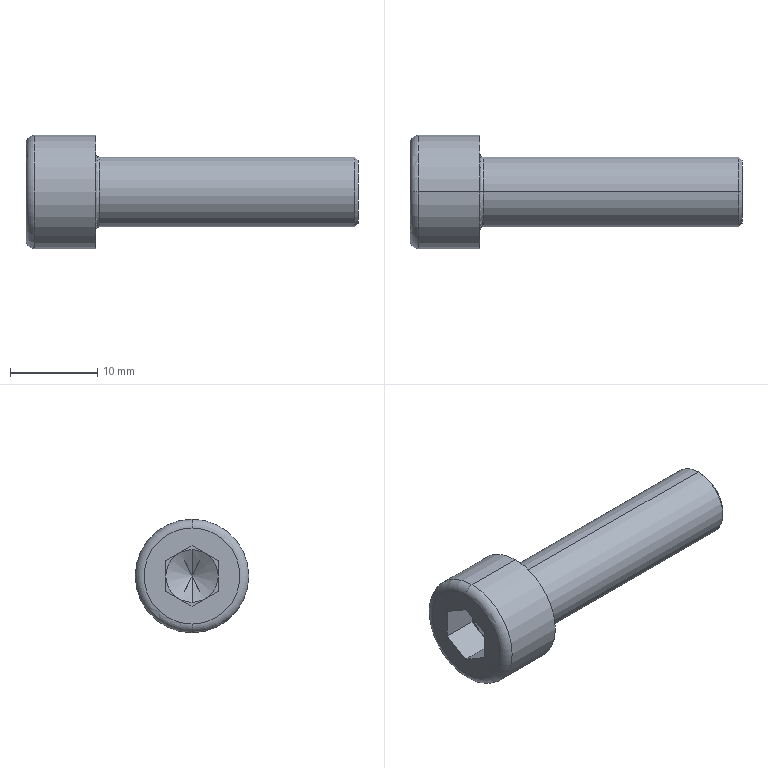Part | SolidWorks | features BaseBody 1 | 1 solid | 27 faces | box 38 x 13 x 13 mm | volume 2419 mm3 | plane 15 | cylinder 4 | torus 4 | cone 4 | commonest cylinder face diameters 8 x2 13 x2
STEP:
#1=CARTESIAN_POINT('',(37.6,0.,4.));
#2=VERTEX_POINT('',#1);
#3=CARTESIAN_POINT('',(37.6,0.,-4.));
#4=VERTEX_POINT('',#3);
#5=CARTESIAN_POINT('',(37.6,0.,0.));
#6=DIRECTION('',(-1.,0.,0.));
#7=DIRECTION('',(0.,0.,1.));
#8=AXIS2_PLACEMENT_3D('',#5,#6,#7);
#9=CIRCLE('',#8,4.);
#10=EDGE_CURVE('',#2,#4,#9,.T.);
#11=ORIENTED_EDGE('',*,*,#10,.T.);
#12=CARTESIAN_POINT('',(8.4,0.,-4.));
#13=VERTEX_POINT('',#12);
#14=CARTESIAN_POINT('',(38.,0.,-4.));
#15=DIRECTION('',(-1.,0.,0.));
#16=VECTOR('',#15,1000.);
#17=LINE('',#14,#16);
#18=EDGE_CURVE('',#4,#13,#17,.T.);
#19=ORIENTED_EDGE('',*,*,#18,.T.);
#20=CARTESIAN_POINT('',(8.4,0.,4.));
#21=VERTEX_POINT('',#20);
#22=CARTESIAN_POINT('',(8.4,0.,0.));
#23=DIRECTION('',(1.,0.,0.));
#24=DIRECTION('',(0.,0.,1.));
#25=AXIS2_PLACEMENT_3D('',#22,#23,#24);
#26=CIRCLE('',#25,4.);
#27=EDGE_CURVE('',#13,#21,#26,.T.);
#28=ORIENTED_EDGE('',*,*,#27,.T.);
#29=CARTESIAN_POINT('',(38.,0.,4.));
#30=DIRECTION('',(-1.,0.,0.));
#31=VECTOR('',#30,1000.);
#32=LINE('',#29,#31);
#33=EDGE_CURVE('',#2,#21,#32,.T.);
#34=ORIENTED_EDGE('',*,*,#33,.F.);
#35=EDGE_LOOP('',(#11,#19,#28,#34));
#36=FACE_OUTER_BOUND('',#35,.T.);
#37=CARTESIAN_POINT('',(38.,0.,0.));
#38=DIRECTION('',(-1.,0.,0.));
#39=DIRECTION('',(0.,0.,1.));
#40=AXIS2_PLACEMENT_3D('',#37,#38,#39);
#41=CYLINDRICAL_SURFACE('',#40,4.);
#42=ADVANCED_FACE('',(#36),#41,.T.);
#43=CARTESIAN_POINT('',(8.4,0.,0.));
#44=DIRECTION('',(1.,0.,0.));
#45=DIRECTION('',(0.,0.,1.));
#46=AXIS2_PLACEMENT_3D('',#43,#44,#45);
#47=CIRCLE('',#46,4.);
#48=EDGE_CURVE('',#21,#13,#47,.T.);
#49=ORIENTED_EDGE('',*,*,#48,.F.);
#50=CARTESIAN_POINT('',(8.,0.,4.4));
#51=VERTEX_POINT('',#50);
#52=CARTESIAN_POINT('',(8.4,0.,4.4));
#53=DIRECTION('',(0.,1.,0.));
#54=DIRECTION('',(0.,0.,1.));
#55=AXIS2_PLACEMENT_3D('',#52,#53,#54);
#56=CIRCLE('',#55,0.4);
#57=EDGE_CURVE('',#21,#51,#56,.T.);
#58=ORIENTED_EDGE('',*,*,#57,.T.);
#59=CARTESIAN_POINT('',(8.,0.,-4.4));
#60=VERTEX_POINT('',#59);
#61=CARTESIAN_POINT('',(8.,0.,-4.4));
#62=CARTESIAN_POINT('',(8.,-0.2798,-4.4));
#63=CARTESIAN_POINT('',(8.,-0.692,-4.361));
#64=CARTESIAN_POINT('',(8.,-1.16,-4.249));
#65=CARTESIAN_POINT('',(8.,-1.391,-4.175));
#66=CARTESIAN_POINT('',(8.,-1.489,-4.141));
#67=CARTESIAN_POINT('',(8.,-1.555,-4.116));
#68=CARTESIAN_POINT('',(8.,-1.585,-4.105));
#69=CARTESIAN_POINT('',(8.,-1.758,-4.036));
#70=CARTESIAN_POINT('',(8.,-1.96,-3.945));
#71=CARTESIAN_POINT('',(8.,-2.154,-3.837));
#72=CARTESIAN_POINT('',(8.,-2.282,-3.763));
#73=CARTESIAN_POINT('',(8.,-2.344,-3.724));
#74=CARTESIAN_POINT('',(8.,-2.661,-3.517));
#75=CARTESIAN_POINT('',(8.,-2.897,-3.326));
#76=CARTESIAN_POINT('',(8.,-3.218,-3.004));
#77=CARTESIAN_POINT('',(8.,-3.37,-2.836));
#78=CARTESIAN_POINT('',(8.,-3.509,-2.656));
#79=CARTESIAN_POINT('',(8.,-3.598,-2.534));
#80=CARTESIAN_POINT('',(8.,-3.642,-2.47));
#81=CARTESIAN_POINT('',(8.,-3.764,-2.284));
#82=CARTESIAN_POINT('',(8.,-3.876,-2.092));
#83=CARTESIAN_POINT('',(8.,-3.989,-1.859));
#84=CARTESIAN_POINT('',(8.,-4.042,-1.74));
#85=CARTESIAN_POINT('',(8.,-4.063,-1.689));
#86=CARTESIAN_POINT('',(8.,-4.077,-1.654));
#87=CARTESIAN_POINT('',(8.,-4.085,-1.636));
#88=CARTESIAN_POINT('',(8.,-4.297,-1.1));
#89=CARTESIAN_POINT('',(8.,-4.4,-0.5588));
#90=CARTESIAN_POINT('',(8.,-4.4,0.2794));
#91=CARTESIAN_POINT('',(8.,-4.361,0.6914));
#92=CARTESIAN_POINT('',(8.,-4.249,1.16));
#93=CARTESIAN_POINT('',(8.,-4.176,1.391));
#94=CARTESIAN_POINT('',(8.,-4.141,1.489));
#95=CARTESIAN_POINT('',(8.,-4.116,1.554));
#96=CARTESIAN_POINT('',(8.,-4.105,1.585));
#97=CARTESIAN_POINT('',(8.,-4.036,1.758));
#98=CARTESIAN_POINT('',(8.,-3.945,1.96));
#99=CARTESIAN_POINT('',(8.,-3.837,2.154));
#100=CARTESIAN_POINT('',(8.,-3.763,2.282));
#101=CARTESIAN_POINT('',(8.,-3.724,2.344));
#102=CARTESIAN_POINT('',(8.,-3.517,2.661));
#103=CARTESIAN_POINT('',(8.,-3.326,2.897));
#104=CARTESIAN_POINT('',(8.,-3.004,3.218));
#105=CARTESIAN_POINT('',(8.,-2.836,3.37));
#106=CARTESIAN_POINT('',(8.,-2.656,3.509));
#107=CARTESIAN_POINT('',(8.,-2.534,3.598));
#108=CARTESIAN_POINT('',(8.,-2.47,3.642));
#109=CARTESIAN_POINT('',(8.,-2.284,3.764));
#110=CARTESIAN_POINT('',(8.,-2.092,3.876));
#111=CARTESIAN_POINT('',(8.,-1.859,3.989));
#112=CARTESIAN_POINT('',(8.,-1.74,4.042));
#113=CARTESIAN_POINT('',(8.,-1.689,4.063));
#114=CARTESIAN_POINT('',(8.,-1.654,4.077));
#115=CARTESIAN_POINT('',(8.,-1.636,4.085));
#116=CARTESIAN_POINT('',(8.,-1.1,4.297));
#117=CARTESIAN_POINT('',(8.,-0.5602,4.4));
#118=CARTESIAN_POINT('',(8.,0.,4.4));
#119=B_SPLINE_CURVE_WITH_KNOTS('',3,(#61,#62,#63,#64,#65,#66,#67,#68,#69,#70,#71,#72,#73,#74,#75,#76,#77,#78,#79,#80,#81,#82,#83,#84,#85,#86,#87,#88,#89,#90,#91,#92,#93,#94,#95,#96,#97,#98,#99,#100,#101,#102,#103,#104,#105,#106,#107,#108,#109,#110,#111,#112,#113,#114,#115,#116,#117,#118),.UNSPECIFIED.,.F.,.F.,(4,1,1,1,2,2,1,2,2,2,1,2,2,1,1,1,2,2,2,1,1,1,2,2,1,2,2,2,1,2,2,1,1,1,2,2,4),(0.,0.0625,0.09375,0.1094,0.1172,0.125,0.1563,0.1719,0.1875,0.25,0.2813,0.2969,0.3125,0.3438,0.3594,0.3672,0.3711,0.375,0.5,0.5625,0.5937,0.6094,0.6172,0.625,0.6562,0.6719,0.6875,0.75,0.7813,0.7969,0.8125,0.8438,0.8594,0.8672,0.8711,0.875,1.),.UNSPECIFIED.);
#120=EDGE_CURVE('',#60,#51,#119,.T.);
#121=ORIENTED_EDGE('',*,*,#120,.F.);
#122=CARTESIAN_POINT('',(8.4,0.,-4.4));
#123=DIRECTION('',(0.,-1.,0.));
#124=DIRECTION('',(0.,0.,-1.));
#125=AXIS2_PLACEMENT_3D('',#122,#123,#124);
#126=CIRCLE('',#125,0.4);
#127=EDGE_CURVE('',#13,#60,#126,.T.);
#128=ORIENTED_EDGE('',*,*,#127,.F.);
#129=EDGE_LOOP('',(#49,#58,#121,#128));
#130=FACE_OUTER_BOUND('',#129,.T.);
#131=CARTESIAN_POINT('',(8.4,0.,0.));
#132=DIRECTION('',(1.,0.,0.));
#133=DIRECTION('',(0.,0.,-1.));
#134=AXIS2_PLACEMENT_3D('',#131,#132,#133);
#135=TOROIDAL_SURFACE('',#134,4.4,0.4);
#136=ADVANCED_FACE('',(#130),#135,.F.);
#137=CARTESIAN_POINT('',(38.,0.,3.6));
#138=VERTEX_POINT('',#137);
#139=CARTESIAN_POINT('',(38.,0.,-3.6));
#140=VERTEX_POINT('',#139);
#141=CARTESIAN_POINT('',(38.,0.,0.));
#142=DIRECTION('',(-1.,0.,0.));
#143=DIRECTION('',(0.,0.,1.));
#144=AXIS2_PLACEMENT_3D('',#141,#142,#143);
#145=CIRCLE('',#144,3.6);
#146=EDGE_CURVE('',#138,#140,#145,.T.);
#147=ORIENTED_EDGE('',*,*,#146,.T.);
#148=CARTESIAN_POINT('',(37.6,0.,-4.));
#149=DIRECTION('',(-0.7071,0.,-0.7071));
#150=VECTOR('',#149,1000.);
#151=LINE('',#148,#150);
#152=EDGE_CURVE('',#140,#4,#151,.T.);
#153=ORIENTED_EDGE('',*,*,#152,.T.);
#154=ORIENTED_EDGE('',*,*,#10,.F.);
#155=CARTESIAN_POINT('',(37.6,0.,4.));
#156=DIRECTION('',(-0.7071,0.,0.7071));
#157=VECTOR('',#156,1000.);
#158=LINE('',#155,#157);
#159=EDGE_CURVE('',#138,#2,#158,.T.);
#160=ORIENTED_EDGE('',*,*,#159,.F.);
#161=EDGE_LOOP('',(#147,#153,#154,#160));
#162=FACE_OUTER_BOUND('',#161,.T.);
#163=CARTESIAN_POINT('',(37.6,0.,0.));
#164=DIRECTION('',(-1.,0.,0.));
#165=DIRECTION('',(0.,0.,1.));
#166=AXIS2_PLACEMENT_3D('',#163,#164,#165);
#167=CONICAL_SURFACE('',#166,4.,0.7854);
#168=ADVANCED_FACE('',(#162),#167,.T.);
#169=CARTESIAN_POINT('',(8.,0.,-6.5));
#170=VERTEX_POINT('',#169);
#171=CARTESIAN_POINT('',(8.,0.,6.5));
#172=VERTEX_POINT('',#171);
#173=CARTESIAN_POINT('',(8.,0.,0.));
#174=DIRECTION('',(1.,0.,0.));
#175=DIRECTION('',(0.,0.,1.));
#176=AXIS2_PLACEMENT_3D('',#173,#174,#175);
#177=CIRCLE('',#176,6.5);
#178=EDGE_CURVE('',#170,#172,#177,.T.);
#179=ORIENTED_EDGE('',*,*,#178,.F.);
#180=CARTESIAN_POINT('',(1.,0.,-6.5));
#181=VERTEX_POINT('',#180);
#182=CARTESIAN_POINT('',(8.,0.,-6.5));
#183=DIRECTION('',(-1.,0.,0.));
#184=VECTOR('',#183,1000.);
#185=LINE('',#182,#184);
#186=EDGE_CURVE('',#170,#181,#185,.T.);
#187=ORIENTED_EDGE('',*,*,#186,.T.);
#188=CARTESIAN_POINT('',(1.,0.,6.5));
#189=VERTEX_POINT('',#188);
#190=CARTESIAN_POINT('',(1.,0.,0.));
#191=DIRECTION('',(1.,0.,0.));
#192=DIRECTION('',(0.,0.,1.));
#193=AXIS2_PLACEMENT_3D('',#190,#191,#192);
#194=CIRCLE('',#193,6.5);
#195=EDGE_CURVE('',#181,#189,#194,.T.);
#196=ORIENTED_EDGE('',*,*,#195,.T.);
#197=CARTESIAN_POINT('',(8.,0.,6.5));
#198=DIRECTION('',(-1.,0.,0.));
#199=VECTOR('',#198,1000.);
#200=LINE('',#197,#199);
#201=EDGE_CURVE('',#172,#189,#200,.T.);
#202=ORIENTED_EDGE('',*,*,#201,.F.);
#203=EDGE_LOOP('',(#179,#187,#196,#202));
#204=FACE_OUTER_BOUND('',#203,.T.);
#205=CARTESIAN_POINT('',(8.,0.,0.));
#206=DIRECTION('',(-1.,0.,0.));
#207=DIRECTION('',(0.,0.,1.));
#208=AXIS2_PLACEMENT_3D('',#205,#206,#207);
#209=CYLINDRICAL_SURFACE('',#208,6.5);
#210=ADVANCED_FACE('',(#204),#209,.T.);
#211=CARTESIAN_POINT('',(0.,0.,-5.5));
#212=VERTEX_POINT('',#211);
#213=CARTESIAN_POINT('',(0.,0.,5.5));
#214=VERTEX_POINT('',#213);
#215=CARTESIAN_POINT('',(0.,0.,0.));
#216=DIRECTION('',(1.,0.,0.));
#217=DIRECTION('',(0.,0.,-1.));
#218=AXIS2_PLACEMENT_3D('',#215,#216,#217);
#219=CIRCLE('',#218,5.5);
#220=EDGE_CURVE('',#212,#214,#219,.T.);
#221=ORIENTED_EDGE('',*,*,#220,.T.);
#222=CARTESIAN_POINT('',(1.,0.,5.5));
#223=DIRECTION('',(0.,1.,0.));
#224=DIRECTION('',(0.,0.,1.));
#225=AXIS2_PLACEMENT_3D('',#222,#223,#224);
#226=CIRCLE('',#225,1.);
#227=EDGE_CURVE('',#214,#189,#226,.T.);
#228=ORIENTED_EDGE('',*,*,#227,.T.);
#229=ORIENTED_EDGE('',*,*,#195,.F.);
#230=CARTESIAN_POINT('',(1.,0.,-5.5));
#231=DIRECTION('',(0.,-1.,0.));
#232=DIRECTION('',(0.,0.,-1.));
#233=AXIS2_PLACEMENT_3D('',#230,#231,#232);
#234=CIRCLE('',#233,1.);
#235=EDGE_CURVE('',#212,#181,#234,.T.);
#236=ORIENTED_EDGE('',*,*,#235,.F.);
#237=EDGE_LOOP('',(#221,#228,#229,#236));
#238=FACE_OUTER_BOUND('',#237,.T.);
#239=CARTESIAN_POINT('',(1.,0.,0.));
#240=DIRECTION('',(1.,0.,0.));
#241=DIRECTION('',(0.,0.,-1.));
#242=AXIS2_PLACEMENT_3D('',#239,#240,#241);
#243=TOROIDAL_SURFACE('',#242,5.5,1.);
#244=ADVANCED_FACE('',(#238),#243,.T.);
#245=CARTESIAN_POINT('',(5.732,0.,0.));
#246=VERTEX_POINT('',#245);
#247=CARTESIAN_POINT('',(4.,0.,3.));
#248=VERTEX_POINT('',#247);
#249=CARTESIAN_POINT('',(4.,0.,3.));
#250=DIRECTION('',(-0.5,0.,0.866));
#251=VECTOR('',#250,1000.);
#252=LINE('',#249,#251);
#253=EDGE_CURVE('',#246,#248,#252,.T.);
#254=ORIENTED_EDGE('',*,*,#253,.F.);
#255=CARTESIAN_POINT('',(4.,0.,-3.));
#256=VERTEX_POINT('',#255);
#257=CARTESIAN_POINT('',(4.,0.,-3.));
#258=DIRECTION('',(-0.5,0.,-0.866));
#259=VECTOR('',#258,1000.);
#260=LINE('',#257,#259);
#261=EDGE_CURVE('',#246,#256,#260,.T.);
#262=ORIENTED_EDGE('',*,*,#261,.T.);
#263=CARTESIAN_POINT('',(4.,-1.5,-2.598));
#264=VERTEX_POINT('',#263);
#265=CARTESIAN_POINT('',(4.,0.,0.));
#266=DIRECTION('',(1.,0.,0.));
#267=DIRECTION('',(0.,0.,1.));
#268=AXIS2_PLACEMENT_3D('',#265,#266,#267);
#269=CIRCLE('',#268,3.);
#270=EDGE_CURVE('',#264,#256,#269,.T.);
#271=ORIENTED_EDGE('',*,*,#270,.F.);
#272=CARTESIAN_POINT('',(4.,-3.,0.));
#273=VERTEX_POINT('',#272);
#274=CARTESIAN_POINT('',(4.,0.,0.));
#275=DIRECTION('',(-1.,0.,0.));
#276=DIRECTION('',(0.,0.,1.));
#277=AXIS2_PLACEMENT_3D('',#274,#275,#276);
#278=CIRCLE('',#277,3.);
#279=EDGE_CURVE('',#264,#273,#278,.T.);
#280=ORIENTED_EDGE('',*,*,#279,.T.);
#281=CARTESIAN_POINT('',(4.,-1.5,2.598));
#282=VERTEX_POINT('',#281);
#283=CARTESIAN_POINT('',(4.,0.,0.));
#284=DIRECTION('',(1.,0.,0.));
#285=DIRECTION('',(0.,0.,1.));
#286=AXIS2_PLACEMENT_3D('',#283,#284,#285);
#287=CIRCLE('',#286,3.);
#288=EDGE_CURVE('',#282,#273,#287,.T.);
#289=ORIENTED_EDGE('',*,*,#288,.F.);
#290=CARTESIAN_POINT('',(4.,0.,0.));
#291=DIRECTION('',(1.,0.,0.));
#292=DIRECTION('',(0.,0.,1.));
#293=AXIS2_PLACEMENT_3D('',#290,#291,#292);
#294=CIRCLE('',#293,3.);
#295=EDGE_CURVE('',#248,#282,#294,.T.);
#296=ORIENTED_EDGE('',*,*,#295,.F.);
#297=EDGE_LOOP('',(#254,#262,#271,#280,#289,#296));
#298=FACE_OUTER_BOUND('',#297,.T.);
#299=CARTESIAN_POINT('',(4.,0.,0.));
#300=DIRECTION('',(-1.,0.,0.));
#301=DIRECTION('',(0.,0.,1.));
#302=AXIS2_PLACEMENT_3D('',#299,#300,#301);
#303=CONICAL_SURFACE('',#302,3.,1.047);
#304=ADVANCED_FACE('',(#298),#303,.F.);
#305=ORIENTED_EDGE('',*,*,#18,.F.);
#306=CARTESIAN_POINT('',(37.6,0.,0.));
#307=DIRECTION('',(-1.,0.,0.));
#308=DIRECTION('',(0.,0.,1.));
#309=AXIS2_PLACEMENT_3D('',#306,#307,#308);
#310=CIRCLE('',#309,4.);
#311=EDGE_CURVE('',#4,#2,#310,.T.);
#312=ORIENTED_EDGE('',*,*,#311,.T.);
#313=ORIENTED_EDGE('',*,*,#33,.T.);
#314=ORIENTED_EDGE('',*,*,#48,.T.);
#315=EDGE_LOOP('',(#305,#312,#313,#314));
#316=FACE_OUTER_BOUND('',#315,.T.);
#317=CARTESIAN_POINT('',(38.,0.,0.));
#318=DIRECTION('',(-1.,0.,0.));
#319=DIRECTION('',(0.,0.,1.));
#320=AXIS2_PLACEMENT_3D('',#317,#318,#319);
#321=CYLINDRICAL_SURFACE('',#320,4.);
#322=ADVANCED_FACE('',(#316),#321,.T.);
#323=ORIENTED_EDGE('',*,*,#57,.F.);
#324=ORIENTED_EDGE('',*,*,#27,.F.);
#325=ORIENTED_EDGE('',*,*,#127,.T.);
#326=CARTESIAN_POINT('',(8.,0.,4.4));
#327=CARTESIAN_POINT('',(8.,0.2798,4.4));
#328=CARTESIAN_POINT('',(8.,0.692,4.361));
#329=CARTESIAN_POINT('',(8.,1.16,4.249));
#330=CARTESIAN_POINT('',(8.,1.391,4.175));
#331=CARTESIAN_POINT('',(8.,1.489,4.141));
#332=CARTESIAN_POINT('',(8.,1.555,4.116));
#333=CARTESIAN_POINT('',(8.,1.585,4.105));
#334=CARTESIAN_POINT('',(8.,1.758,4.036));
#335=CARTESIAN_POINT('',(8.,1.96,3.945));
#336=CARTESIAN_POINT('',(8.,2.154,3.837));
#337=CARTESIAN_POINT('',(8.,2.282,3.763));
#338=CARTESIAN_POINT('',(8.,2.344,3.724));
#339=CARTESIAN_POINT('',(8.,2.661,3.517));
#340=CARTESIAN_POINT('',(8.,2.897,3.326));
#341=CARTESIAN_POINT('',(8.,3.218,3.004));
#342=CARTESIAN_POINT('',(8.,3.37,2.836));
#343=CARTESIAN_POINT('',(8.,3.509,2.656));
#344=CARTESIAN_POINT('',(8.,3.598,2.534));
#345=CARTESIAN_POINT('',(8.,3.642,2.47));
#346=CARTESIAN_POINT('',(8.,3.764,2.284));
#347=CARTESIAN_POINT('',(8.,3.876,2.092));
#348=CARTESIAN_POINT('',(8.,3.989,1.859));
#349=CARTESIAN_POINT('',(8.,4.042,1.74));
#350=CARTESIAN_POINT('',(8.,4.063,1.689));
#351=CARTESIAN_POINT('',(8.,4.077,1.654));
#352=CARTESIAN_POINT('',(8.,4.085,1.636));
#353=CARTESIAN_POINT('',(8.,4.297,1.1));
#354=CARTESIAN_POINT('',(8.,4.4,0.5588));
#355=CARTESIAN_POINT('',(8.,4.4,-0.2794));
#356=CARTESIAN_POINT('',(8.,4.361,-0.6914));
#357=CARTESIAN_POINT('',(8.,4.249,-1.16));
#358=CARTESIAN_POINT('',(8.,4.176,-1.391));
#359=CARTESIAN_POINT('',(8.,4.141,-1.489));
#360=CARTESIAN_POINT('',(8.,4.116,-1.554));
#361=CARTESIAN_POINT('',(8.,4.105,-1.585));
#362=CARTESIAN_POINT('',(8.,4.036,-1.758));
#363=CARTESIAN_POINT('',(8.,3.945,-1.96));
#364=CARTESIAN_POINT('',(8.,3.837,-2.154));
#365=CARTESIAN_POINT('',(8.,3.763,-2.282));
#366=CARTESIAN_POINT('',(8.,3.724,-2.344));
#367=CARTESIAN_POINT('',(8.,3.517,-2.661));
#368=CARTESIAN_POINT('',(8.,3.326,-2.897));
#369=CARTESIAN_POINT('',(8.,3.004,-3.218));
#370=CARTESIAN_POINT('',(8.,2.836,-3.37));
#371=CARTESIAN_POINT('',(8.,2.656,-3.509));
#372=CARTESIAN_POINT('',(8.,2.534,-3.598));
#373=CARTESIAN_POINT('',(8.,2.47,-3.642));
#374=CARTESIAN_POINT('',(8.,2.284,-3.764));
#375=CARTESIAN_POINT('',(8.,2.092,-3.876));
#376=CARTESIAN_POINT('',(8.,1.859,-3.989));
#377=CARTESIAN_POINT('',(8.,1.74,-4.042));
#378=CARTESIAN_POINT('',(8.,1.689,-4.063));
#379=CARTESIAN_POINT('',(8.,1.654,-4.077));
#380=CARTESIAN_POINT('',(8.,1.636,-4.085));
#381=CARTESIAN_POINT('',(8.,1.1,-4.297));
#382=CARTESIAN_POINT('',(8.,0.5602,-4.4));
#383=CARTESIAN_POINT('',(8.,0.,-4.4));
#384=B_SPLINE_CURVE_WITH_KNOTS('',3,(#326,#327,#328,#329,#330,#331,#332,#333,#334,#335,#336,#337,#338,#339,#340,#341,#342,#343,#344,#345,#346,#347,#348,#349,#350,#351,#352,#353,#354,#355,#356,#357,#358,#359,#360,#361,#362,#363,#364,#365,#366,#367,#368,#369,#370,#371,#372,#373,#374,#375,#376,#377,#378,#379,#380,#381,#382,#383),.UNSPECIFIED.,.F.,.F.,(4,1,1,1,2,2,1,2,2,2,1,2,2,1,1,1,2,2,2,1,1,1,2,2,1,2,2,2,1,2,2,1,1,1,2,2,4),(0.,0.0625,0.09375,0.1094,0.1172,0.125,0.1563,0.1719,0.1875,0.25,0.2813,0.2969,0.3125,0.3438,0.3594,0.3672,0.3711,0.375,0.5,0.5625,0.5937,0.6094,0.6172,0.625,0.6562,0.6719,0.6875,0.75,0.7812,0.7969,0.8125,0.8437,0.8594,0.8672,0.8711,0.875,1.),.UNSPECIFIED.);
#385=EDGE_CURVE('',#51,#60,#384,.T.);
#386=ORIENTED_EDGE('',*,*,#385,.F.);
#387=EDGE_LOOP('',(#323,#324,#325,#386));
#388=FACE_OUTER_BOUND('',#387,.T.);
#389=CARTESIAN_POINT('',(8.4,0.,0.));
#390=DIRECTION('',(1.,0.,0.));
#391=DIRECTION('',(0.,0.,-1.));
#392=AXIS2_PLACEMENT_3D('',#389,#390,#391);
#393=TOROIDAL_SURFACE('',#392,4.4,0.4);
#394=ADVANCED_FACE('',(#388),#393,.F.);
#395=ORIENTED_EDGE('',*,*,#152,.F.);
#396=CARTESIAN_POINT('',(38.,0.,0.));
#397=DIRECTION('',(-1.,0.,0.));
#398=DIRECTION('',(0.,0.,1.));
#399=AXIS2_PLACEMENT_3D('',#396,#397,#398);
#400=CIRCLE('',#399,3.6);
#401=EDGE_CURVE('',#140,#138,#400,.T.);
#402=ORIENTED_EDGE('',*,*,#401,.T.);
#403=ORIENTED_EDGE('',*,*,#159,.T.);
#404=ORIENTED_EDGE('',*,*,#311,.F.);
#405=EDGE_LOOP('',(#395,#402,#403,#404));
#406=FACE_OUTER_BOUND('',#405,.T.);
#407=CARTESIAN_POINT('',(37.6,0.,0.));
#408=DIRECTION('',(-1.,0.,0.));
#409=DIRECTION('',(0.,0.,1.));
#410=AXIS2_PLACEMENT_3D('',#407,#408,#409);
#411=CONICAL_SURFACE('',#410,4.,0.7854);
#412=ADVANCED_FACE('',(#406),#411,.T.);
#413=ORIENTED_EDGE('',*,*,#120,.T.);
#414=ORIENTED_EDGE('',*,*,#385,.T.);
#415=EDGE_LOOP('',(#413,#414));
#416=FACE_BOUND('',#415,.T.);
#417=CARTESIAN_POINT('',(8.,0.,0.));
#418=DIRECTION('',(1.,0.,0.));
#419=DIRECTION('',(0.,0.,1.));
#420=AXIS2_PLACEMENT_3D('',#417,#418,#419);
#421=CIRCLE('',#420,6.5);
#422=EDGE_CURVE('',#172,#170,#421,.T.);
#423=ORIENTED_EDGE('',*,*,#422,.T.);
#424=ORIENTED_EDGE('',*,*,#178,.T.);
#425=EDGE_LOOP('',(#423,#424));
#426=FACE_OUTER_BOUND('',#425,.T.);
#427=CARTESIAN_POINT('',(8.,0.,0.));
#428=DIRECTION('',(1.,0.,0.));
#429=DIRECTION('',(0.,0.,-1.));
#430=AXIS2_PLACEMENT_3D('',#427,#428,#429);
#431=PLANE('',#430);
#432=ADVANCED_FACE('',(#416,#426),#431,.T.);
#433=ORIENTED_EDGE('',*,*,#146,.F.);
#434=ORIENTED_EDGE('',*,*,#401,.F.);
#435=EDGE_LOOP('',(#433,#434));
#436=FACE_OUTER_BOUND('',#435,.T.);
#437=CARTESIAN_POINT('',(38.,0.,0.));
#438=DIRECTION('',(1.,0.,0.));
#439=DIRECTION('',(0.,0.,-1.));
#440=AXIS2_PLACEMENT_3D('',#437,#438,#439);
#441=PLANE('',#440);
#442=ADVANCED_FACE('',(#436),#441,.T.);
#443=ORIENTED_EDGE('',*,*,#186,.F.);
#444=ORIENTED_EDGE('',*,*,#422,.F.);
#445=ORIENTED_EDGE('',*,*,#201,.T.);
#446=CARTESIAN_POINT('',(1.,0.,0.));
#447=DIRECTION('',(1.,0.,0.));
#448=DIRECTION('',(0.,0.,1.));
#449=AXIS2_PLACEMENT_3D('',#446,#447,#448);
#450=CIRCLE('',#449,6.5);
#451=EDGE_CURVE('',#189,#181,#450,.T.);
#452=ORIENTED_EDGE('',*,*,#451,.T.);
#453=EDGE_LOOP('',(#443,#444,#445,#452));
#454=FACE_OUTER_BOUND('',#453,.T.);
#455=CARTESIAN_POINT('',(8.,0.,0.));
#456=DIRECTION('',(-1.,0.,0.));
#457=DIRECTION('',(0.,0.,1.));
#458=AXIS2_PLACEMENT_3D('',#455,#456,#457);
#459=CYLINDRICAL_SURFACE('',#458,6.5);
#460=ADVANCED_FACE('',(#454),#459,.T.);
#461=ORIENTED_EDGE('',*,*,#227,.F.);
#462=CARTESIAN_POINT('',(0.,0.,0.));
#463=DIRECTION('',(1.,0.,0.));
#464=DIRECTION('',(0.,0.,-1.));
#465=AXIS2_PLACEMENT_3D('',#462,#463,#464);
#466=CIRCLE('',#465,5.5);
#467=EDGE_CURVE('',#214,#212,#466,.T.);
#468=ORIENTED_EDGE('',*,*,#467,.T.);
#469=ORIENTED_EDGE('',*,*,#235,.T.);
#470=ORIENTED_EDGE('',*,*,#451,.F.);
#471=EDGE_LOOP('',(#461,#468,#469,#470));
#472=FACE_OUTER_BOUND('',#471,.T.);
#473=CARTESIAN_POINT('',(1.,0.,0.));
#474=DIRECTION('',(1.,0.,0.));
#475=DIRECTION('',(0.,0.,-1.));
#476=AXIS2_PLACEMENT_3D('',#473,#474,#475);
#477=TOROIDAL_SURFACE('',#476,5.5,1.);
#478=ADVANCED_FACE('',(#472),#477,.T.);
#479=ORIENTED_EDGE('',*,*,#220,.F.);
#480=ORIENTED_EDGE('',*,*,#467,.F.);
#481=EDGE_LOOP('',(#479,#480));
#482=FACE_OUTER_BOUND('',#481,.T.);
#483=CARTESIAN_POINT('',(0.,3.,1.732));
#484=VERTEX_POINT('',#483);
#485=CARTESIAN_POINT('',(0.,3.,-1.732));
#486=VERTEX_POINT('',#485);
#487=CARTESIAN_POINT('',(0.,3.,0.));
#488=DIRECTION('',(0.,0.,-1.));
#489=VECTOR('',#488,1000.);
#490=LINE('',#487,#489);
#491=EDGE_CURVE('',#484,#486,#490,.T.);
#492=ORIENTED_EDGE('',*,*,#491,.F.);
#493=CARTESIAN_POINT('',(0.,0.,3.464));
#494=VERTEX_POINT('',#493);
#495=CARTESIAN_POINT('',(0.,0.,3.464));
#496=DIRECTION('',(0.,0.866,-0.5));
#497=VECTOR('',#496,1000.);
#498=LINE('',#495,#497);
#499=EDGE_CURVE('',#494,#484,#498,.T.);
#500=ORIENTED_EDGE('',*,*,#499,.F.);
#501=CARTESIAN_POINT('',(0.,-3.,1.732));
#502=VERTEX_POINT('',#501);
#503=CARTESIAN_POINT('',(0.,-3.,1.732));
#504=DIRECTION('',(0.,0.866,0.5));
#505=VECTOR('',#504,1000.);
#506=LINE('',#503,#505);
#507=EDGE_CURVE('',#502,#494,#506,.T.);
#508=ORIENTED_EDGE('',*,*,#507,.F.);
#509=CARTESIAN_POINT('',(0.,-3.,-1.732));
#510=VERTEX_POINT('',#509);
#511=CARTESIAN_POINT('',(0.,-3.,0.));
#512=DIRECTION('',(0.,0.,1.));
#513=VECTOR('',#512,1000.);
#514=LINE('',#511,#513);
#515=EDGE_CURVE('',#510,#502,#514,.T.);
#516=ORIENTED_EDGE('',*,*,#515,.F.);
#517=CARTESIAN_POINT('',(0.,0.,-3.464));
#518=VERTEX_POINT('',#517);
#519=CARTESIAN_POINT('',(0.,0.,-3.464));
#520=DIRECTION('',(0.,-0.866,0.5));
#521=VECTOR('',#520,1000.);
#522=LINE('',#519,#521);
#523=EDGE_CURVE('',#518,#510,#522,.T.);
#524=ORIENTED_EDGE('',*,*,#523,.F.);
#525=CARTESIAN_POINT('',(0.,3.,-1.732));
#526=DIRECTION('',(0.,-0.866,-0.5));
#527=VECTOR('',#526,1000.);
#528=LINE('',#525,#527);
#529=EDGE_CURVE('',#486,#518,#528,.T.);
#530=ORIENTED_EDGE('',*,*,#529,.F.);
#531=EDGE_LOOP('',(#492,#500,#508,#516,#524,#530));
#532=FACE_BOUND('',#531,.T.);
#533=CARTESIAN_POINT('',(0.,0.,0.));
#534=DIRECTION('',(1.,0.,0.));
#535=DIRECTION('',(0.,0.,-1.));
#536=AXIS2_PLACEMENT_3D('',#533,#534,#535);
#537=PLANE('',#536);
#538=ADVANCED_FACE('',(#482,#532),#537,.F.);
#539=CARTESIAN_POINT('',(4.,0.,-3.464));
#540=VERTEX_POINT('',#539);
#541=CARTESIAN_POINT('',(4.,0.,-3.464));
#542=DIRECTION('',(1.,0.,0.));
#543=VECTOR('',#542,1000.);
#544=LINE('',#541,#543);
#545=EDGE_CURVE('',#518,#540,#544,.T.);
#546=ORIENTED_EDGE('',*,*,#545,.T.);
#547=CARTESIAN_POINT('',(4.,1.5,-2.598));
#548=VERTEX_POINT('',#547);
#549=CARTESIAN_POINT('',(4.,0.,-3.464));
#550=DIRECTION('',(0.,0.866,0.5));
#551=VECTOR('',#550,1000.);
#552=LINE('',#549,#551);
#553=EDGE_CURVE('',#540,#548,#552,.T.);
#554=ORIENTED_EDGE('',*,*,#553,.T.);
#555=CARTESIAN_POINT('',(4.,3.,-1.732));
#556=VERTEX_POINT('',#555);
#557=CARTESIAN_POINT('',(4.,1.5,-2.598));
#558=DIRECTION('',(0.,0.866,0.5));
#559=VECTOR('',#558,1000.);
#560=LINE('',#557,#559);
#561=EDGE_CURVE('',#548,#556,#560,.T.);
#562=ORIENTED_EDGE('',*,*,#561,.T.);
#563=CARTESIAN_POINT('',(4.,3.,-1.732));
#564=DIRECTION('',(-1.,0.,0.));
#565=VECTOR('',#564,1000.);
#566=LINE('',#563,#565);
#567=EDGE_CURVE('',#556,#486,#566,.T.);
#568=ORIENTED_EDGE('',*,*,#567,.T.);
#569=ORIENTED_EDGE('',*,*,#529,.T.);
#570=EDGE_LOOP('',(#546,#554,#562,#568,#569));
#571=FACE_OUTER_BOUND('',#570,.T.);
#572=CARTESIAN_POINT('',(4.,0.,-3.464));
#573=DIRECTION('',(0.,-0.5,0.866));
#574=DIRECTION('',(0.,-0.866,-0.5));
#575=AXIS2_PLACEMENT_3D('',#572,#573,#574);
#576=PLANE('',#575);
#577=ADVANCED_FACE('',(#571),#576,.T.);
#578=ORIENTED_EDGE('',*,*,#567,.F.);
#579=CARTESIAN_POINT('',(4.,3.,0.));
#580=VERTEX_POINT('',#579);
#581=CARTESIAN_POINT('',(4.,3.,-3.464));
#582=DIRECTION('',(0.,0.,1.));
#583=VECTOR('',#582,1000.);
#584=LINE('',#581,#583);
#585=EDGE_CURVE('',#556,#580,#584,.T.);
#586=ORIENTED_EDGE('',*,*,#585,.T.);
#587=CARTESIAN_POINT('',(4.,3.,1.732));
#588=VERTEX_POINT('',#587);
#589=CARTESIAN_POINT('',(4.,3.,-3.464));
#590=DIRECTION('',(0.,0.,1.));
#591=VECTOR('',#590,1000.);
#592=LINE('',#589,#591);
#593=EDGE_CURVE('',#580,#588,#592,.T.);
#594=ORIENTED_EDGE('',*,*,#593,.T.);
#595=CARTESIAN_POINT('',(4.,3.,1.732));
#596=DIRECTION('',(-1.,0.,0.));
#597=VECTOR('',#596,1000.);
#598=LINE('',#595,#597);
#599=EDGE_CURVE('',#588,#484,#598,.T.);
#600=ORIENTED_EDGE('',*,*,#599,.T.);
#601=ORIENTED_EDGE('',*,*,#491,.T.);
#602=EDGE_LOOP('',(#578,#586,#594,#600,#601));
#603=FACE_OUTER_BOUND('',#602,.T.);
#604=CARTESIAN_POINT('',(4.,3.,-1.732));
#605=DIRECTION('',(0.,-1.,0.));
#606=DIRECTION('',(0.,0.,-1.));
#607=AXIS2_PLACEMENT_3D('',#604,#605,#606);
#608=PLANE('',#607);
#609=ADVANCED_FACE('',(#603),#608,.T.);
#610=ORIENTED_EDGE('',*,*,#599,.F.);
#611=CARTESIAN_POINT('',(4.,1.5,2.598));
#612=VERTEX_POINT('',#611);
#613=CARTESIAN_POINT('',(4.,3.,1.732));
#614=DIRECTION('',(0.,-0.866,0.5));
#615=VECTOR('',#614,1000.);
#616=LINE('',#613,#615);
#617=EDGE_CURVE('',#588,#612,#616,.T.);
#618=ORIENTED_EDGE('',*,*,#617,.T.);
#619=CARTESIAN_POINT('',(4.,0.,3.464));
#620=VERTEX_POINT('',#619);
#621=CARTESIAN_POINT('',(4.,3.,1.732));
#622=DIRECTION('',(0.,-0.866,0.5));
#623=VECTOR('',#622,1000.);
#624=LINE('',#621,#623);
#625=EDGE_CURVE('',#612,#620,#624,.T.);
#626=ORIENTED_EDGE('',*,*,#625,.T.);
#627=CARTESIAN_POINT('',(4.,0.,3.464));
#628=DIRECTION('',(-1.,0.,0.));
#629=VECTOR('',#628,1000.);
#630=LINE('',#627,#629);
#631=EDGE_CURVE('',#620,#494,#630,.T.);
#632=ORIENTED_EDGE('',*,*,#631,.T.);
#633=ORIENTED_EDGE('',*,*,#499,.T.);
#634=EDGE_LOOP('',(#610,#618,#626,#632,#633));
#635=FACE_OUTER_BOUND('',#634,.T.);
#636=CARTESIAN_POINT('',(4.,3.,1.732));
#637=DIRECTION('',(0.,-0.5,-0.866));
#638=DIRECTION('',(0.,0.866,-0.5));
#639=AXIS2_PLACEMENT_3D('',#636,#637,#638);
#640=PLANE('',#639);
#641=ADVANCED_FACE('',(#635),#640,.T.);
#642=ORIENTED_EDGE('',*,*,#631,.F.);
#643=CARTESIAN_POINT('',(4.,0.,3.464));
#644=DIRECTION('',(0.,-0.866,-0.5));
#645=VECTOR('',#644,1000.);
#646=LINE('',#643,#645);
#647=EDGE_CURVE('',#620,#282,#646,.T.);
#648=ORIENTED_EDGE('',*,*,#647,.T.);
#649=CARTESIAN_POINT('',(4.,-3.,1.732));
#650=VERTEX_POINT('',#649);
#651=CARTESIAN_POINT('',(4.,-1.5,2.598));
#652=DIRECTION('',(0.,-0.866,-0.5));
#653=VECTOR('',#652,1000.);
#654=LINE('',#651,#653);
#655=EDGE_CURVE('',#282,#650,#654,.T.);
#656=ORIENTED_EDGE('',*,*,#655,.T.);
#657=CARTESIAN_POINT('',(4.,-3.,1.732));
#658=DIRECTION('',(-1.,0.,0.));
#659=VECTOR('',#658,1000.);
#660=LINE('',#657,#659);
#661=EDGE_CURVE('',#650,#502,#660,.T.);
#662=ORIENTED_EDGE('',*,*,#661,.T.);
#663=ORIENTED_EDGE('',*,*,#507,.T.);
#664=EDGE_LOOP('',(#642,#648,#656,#662,#663));
#665=FACE_OUTER_BOUND('',#664,.T.);
#666=CARTESIAN_POINT('',(4.,0.,3.464));
#667=DIRECTION('',(0.,0.5,-0.866));
#668=DIRECTION('',(0.,0.866,0.5));
#669=AXIS2_PLACEMENT_3D('',#666,#667,#668);
#670=PLANE('',#669);
#671=ADVANCED_FACE('',(#665),#670,.T.);
#672=ORIENTED_EDGE('',*,*,#661,.F.);
#673=CARTESIAN_POINT('',(4.,-3.,-3.464));
#674=DIRECTION('',(0.,0.,-1.));
#675=VECTOR('',#674,1000.);
#676=LINE('',#673,#675);
#677=EDGE_CURVE('',#650,#273,#676,.T.);
#678=ORIENTED_EDGE('',*,*,#677,.T.);
#679=CARTESIAN_POINT('',(4.,-3.,-1.732));
#680=VERTEX_POINT('',#679);
#681=CARTESIAN_POINT('',(4.,-3.,1.732));
#682=DIRECTION('',(0.,0.,-1.));
#683=VECTOR('',#682,1000.);
#684=LINE('',#681,#683);
#685=EDGE_CURVE('',#273,#680,#684,.T.);
#686=ORIENTED_EDGE('',*,*,#685,.T.);
#687=CARTESIAN_POINT('',(4.,-3.,-1.732));
#688=DIRECTION('',(-1.,0.,0.));
#689=VECTOR('',#688,1000.);
#690=LINE('',#687,#689);
#691=EDGE_CURVE('',#680,#510,#690,.T.);
#692=ORIENTED_EDGE('',*,*,#691,.T.);
#693=ORIENTED_EDGE('',*,*,#515,.T.);
#694=EDGE_LOOP('',(#672,#678,#686,#692,#693));
#695=FACE_OUTER_BOUND('',#694,.T.);
#696=CARTESIAN_POINT('',(4.,-3.,1.732));
#697=DIRECTION('',(0.,1.,0.));
#698=DIRECTION('',(0.,0.,1.));
#699=AXIS2_PLACEMENT_3D('',#696,#697,#698);
#700=PLANE('',#699);
#701=ADVANCED_FACE('',(#695),#700,.T.);
#702=ORIENTED_EDGE('',*,*,#691,.F.);
#703=CARTESIAN_POINT('',(4.,-3.,-1.732));
#704=DIRECTION('',(0.,0.866,-0.5));
#705=VECTOR('',#704,1000.);
#706=LINE('',#703,#705);
#707=EDGE_CURVE('',#680,#264,#706,.T.);
#708=ORIENTED_EDGE('',*,*,#707,.T.);
#709=CARTESIAN_POINT('',(4.,-3.,-1.732));
#710=DIRECTION('',(0.,0.866,-0.5));
#711=VECTOR('',#710,1000.);
#712=LINE('',#709,#711);
#713=EDGE_CURVE('',#264,#540,#712,.T.);
#714=ORIENTED_EDGE('',*,*,#713,.T.);
#715=ORIENTED_EDGE('',*,*,#545,.F.);
#716=ORIENTED_EDGE('',*,*,#523,.T.);
#717=EDGE_LOOP('',(#702,#708,#714,#715,#716));
#718=FACE_OUTER_BOUND('',#717,.T.);
#719=CARTESIAN_POINT('',(4.,-3.,-1.732));
#720=DIRECTION('',(0.,0.5,0.866));
#721=DIRECTION('',(0.,-0.866,0.5));
#722=AXIS2_PLACEMENT_3D('',#719,#720,#721);
#723=PLANE('',#722);
#724=ADVANCED_FACE('',(#718),#723,.T.);
#725=ORIENTED_EDGE('',*,*,#270,.T.);
#726=CARTESIAN_POINT('',(4.,0.,0.));
#727=DIRECTION('',(1.,0.,0.));
#728=DIRECTION('',(0.,0.,1.));
#729=AXIS2_PLACEMENT_3D('',#726,#727,#728);
#730=CIRCLE('',#729,3.);
#731=EDGE_CURVE('',#256,#548,#730,.T.);
#732=ORIENTED_EDGE('',*,*,#731,.T.);
#733=ORIENTED_EDGE('',*,*,#553,.F.);
#734=ORIENTED_EDGE('',*,*,#713,.F.);
#735=EDGE_LOOP('',(#725,#732,#733,#734));
#736=FACE_OUTER_BOUND('',#735,.T.);
#737=CARTESIAN_POINT('',(4.,0.,-3.464));
#738=DIRECTION('',(1.,0.,0.));
#739=DIRECTION('',(0.,0.,-1.));
#740=AXIS2_PLACEMENT_3D('',#737,#738,#739);
#741=PLANE('',#740);
#742=ADVANCED_FACE('',(#736),#741,.F.);
#743=ORIENTED_EDGE('',*,*,#625,.F.);
#744=CARTESIAN_POINT('',(4.,0.,0.));
#745=DIRECTION('',(1.,0.,0.));
#746=DIRECTION('',(0.,0.,1.));
#747=AXIS2_PLACEMENT_3D('',#744,#745,#746);
#748=CIRCLE('',#747,3.);
#749=EDGE_CURVE('',#612,#248,#748,.T.);
#750=ORIENTED_EDGE('',*,*,#749,.T.);
#751=ORIENTED_EDGE('',*,*,#295,.T.);
#752=ORIENTED_EDGE('',*,*,#647,.F.);
#753=EDGE_LOOP('',(#743,#750,#751,#752));
#754=FACE_OUTER_BOUND('',#753,.T.);
#755=CARTESIAN_POINT('',(4.,0.,-3.464));
#756=DIRECTION('',(1.,0.,0.));
#757=DIRECTION('',(0.,0.,-1.));
#758=AXIS2_PLACEMENT_3D('',#755,#756,#757);
#759=PLANE('',#758);
#760=ADVANCED_FACE('',(#754),#759,.F.);
#761=ORIENTED_EDGE('',*,*,#707,.F.);
#762=ORIENTED_EDGE('',*,*,#685,.F.);
#763=ORIENTED_EDGE('',*,*,#279,.F.);
#764=EDGE_LOOP('',(#761,#762,#763));
#765=FACE_OUTER_BOUND('',#764,.T.);
#766=CARTESIAN_POINT('',(4.,0.,-3.464));
#767=DIRECTION('',(1.,0.,0.));
#768=DIRECTION('',(0.,0.,-1.));
#769=AXIS2_PLACEMENT_3D('',#766,#767,#768);
#770=PLANE('',#769);
#771=ADVANCED_FACE('',(#765),#770,.F.);
#772=ORIENTED_EDGE('',*,*,#261,.F.);
#773=ORIENTED_EDGE('',*,*,#253,.T.);
#774=ORIENTED_EDGE('',*,*,#749,.F.);
#775=CARTESIAN_POINT('',(4.,0.,0.));
#776=DIRECTION('',(1.,0.,0.));
#777=DIRECTION('',(0.,0.,1.));
#778=AXIS2_PLACEMENT_3D('',#775,#776,#777);
#779=CIRCLE('',#778,3.);
#780=EDGE_CURVE('',#580,#612,#779,.T.);
#781=ORIENTED_EDGE('',*,*,#780,.F.);
#782=CARTESIAN_POINT('',(4.,0.,0.));
#783=DIRECTION('',(1.,0.,0.));
#784=DIRECTION('',(0.,0.,1.));
#785=AXIS2_PLACEMENT_3D('',#782,#783,#784);
#786=CIRCLE('',#785,3.);
#787=EDGE_CURVE('',#548,#580,#786,.T.);
#788=ORIENTED_EDGE('',*,*,#787,.F.);
#789=ORIENTED_EDGE('',*,*,#731,.F.);
#790=EDGE_LOOP('',(#772,#773,#774,#781,#788,#789));
#791=FACE_OUTER_BOUND('',#790,.T.);
#792=CARTESIAN_POINT('',(4.,0.,0.));
#793=DIRECTION('',(-1.,0.,0.));
#794=DIRECTION('',(0.,0.,1.));
#795=AXIS2_PLACEMENT_3D('',#792,#793,#794);
#796=CONICAL_SURFACE('',#795,3.,1.047);
#797=ADVANCED_FACE('',(#791),#796,.F.);
#798=ORIENTED_EDGE('',*,*,#677,.F.);
#799=ORIENTED_EDGE('',*,*,#655,.F.);
#800=ORIENTED_EDGE('',*,*,#288,.T.);
#801=EDGE_LOOP('',(#798,#799,#800));
#802=FACE_OUTER_BOUND('',#801,.T.);
#803=CARTESIAN_POINT('',(4.,0.,-3.464));
#804=DIRECTION('',(1.,0.,0.));
#805=DIRECTION('',(0.,0.,-1.));
#806=AXIS2_PLACEMENT_3D('',#803,#804,#805);
#807=PLANE('',#806);
#808=ADVANCED_FACE('',(#802),#807,.F.);
#809=ORIENTED_EDGE('',*,*,#617,.F.);
#810=ORIENTED_EDGE('',*,*,#593,.F.);
#811=ORIENTED_EDGE('',*,*,#780,.T.);
#812=EDGE_LOOP('',(#809,#810,#811));
#813=FACE_OUTER_BOUND('',#812,.T.);
#814=CARTESIAN_POINT('',(4.,0.,-3.464));
#815=DIRECTION('',(1.,0.,0.));
#816=DIRECTION('',(0.,0.,-1.));
#817=AXIS2_PLACEMENT_3D('',#814,#815,#816);
#818=PLANE('',#817);
#819=ADVANCED_FACE('',(#813),#818,.F.);
#820=ORIENTED_EDGE('',*,*,#585,.F.);
#821=ORIENTED_EDGE('',*,*,#561,.F.);
#822=ORIENTED_EDGE('',*,*,#787,.T.);
#823=EDGE_LOOP('',(#820,#821,#822));
#824=FACE_OUTER_BOUND('',#823,.T.);
#825=CARTESIAN_POINT('',(4.,0.,-3.464));
#826=DIRECTION('',(1.,0.,0.));
#827=DIRECTION('',(0.,0.,-1.));
#828=AXIS2_PLACEMENT_3D('',#825,#826,#827);
#829=PLANE('',#828);
#830=ADVANCED_FACE('',(#824),#829,.F.);
#831=CLOSED_SHELL('',(#42,#136,#168,#210,#244,#304,#322,#394,#412,#432,#442,#460,#478,#538,#577,#609,#641,#671,#701,#724,#742,#760,#771,#797,#808,#819,#830));
#832=MANIFOLD_SOLID_BREP('',#831);
#833=CARTESIAN_POINT('',(0.,0.,0.));
#834=DIRECTION('',(0.,0.,1.));
#835=DIRECTION('',(1.,0.,0.));
#836=AXIS2_PLACEMENT_3D('',#833,#834,#835);
#837=(LENGTH_UNIT()NAMED_UNIT(*)SI_UNIT(.MILLI.,.METRE.));
#838=UNCERTAINTY_MEASURE_WITH_UNIT(LENGTH_MEASURE(0.00001),#837,'','');
#839=(NAMED_UNIT(*)PLANE_ANGLE_UNIT()SI_UNIT($,.RADIAN.));
#840=(NAMED_UNIT(*)SI_UNIT($,.STERADIAN.)SOLID_ANGLE_UNIT());
#841=(GEOMETRIC_REPRESENTATION_CONTEXT(3)GLOBAL_UNCERTAINTY_ASSIGNED_CONTEXT((#838))GLOBAL_UNIT_ASSIGNED_CONTEXT((#837,#839,#840))REPRESENTATION_CONTEXT('',''));
#842=ADVANCED_BREP_SHAPE_REPRESENTATION('',(#832,#836),#841);